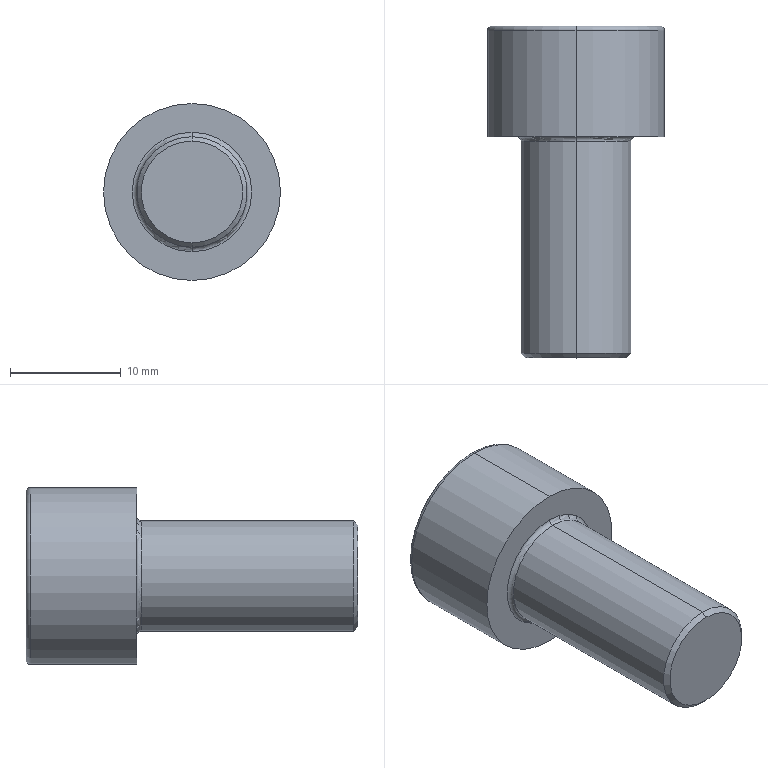Part | STEP file | 1 solid | 20 faces | box 16 x 30 x 16 mm | volume 3301 mm3 | plane 10 | torus 4 | cylinder 4 | cone 2 | commonest cylinder face diameters 10 x2 16 x2
STEP:
#1=CARTESIAN_POINT('',(0.,-20.,-4.6));
#2=VERTEX_POINT('',#1);
#3=CARTESIAN_POINT('',(0.,-20.,4.6));
#4=VERTEX_POINT('',#3);
#5=CARTESIAN_POINT('',(0.,-20.,0.));
#6=DIRECTION('',(0.,-1.,0.));
#7=DIRECTION('',(0.,0.,-1.));
#8=AXIS2_PLACEMENT_3D('',#5,#6,#7);
#9=CIRCLE('',#8,4.6);
#10=EDGE_CURVE('',#2,#4,#9,.T.);
#11=ORIENTED_EDGE('',*,*,#10,.F.);
#12=CARTESIAN_POINT('',(0.,-19.6,-5.));
#13=VERTEX_POINT('',#12);
#14=CARTESIAN_POINT('',(0.,-20.,-4.6));
#15=DIRECTION('',(0.,0.7071,-0.7071));
#16=VECTOR('',#15,1000.);
#17=LINE('',#14,#16);
#18=EDGE_CURVE('',#2,#13,#17,.T.);
#19=ORIENTED_EDGE('',*,*,#18,.T.);
#20=CARTESIAN_POINT('',(0.,-19.6,5.));
#21=VERTEX_POINT('',#20);
#22=CARTESIAN_POINT('',(0.,-19.6,0.));
#23=DIRECTION('',(0.,1.,0.));
#24=DIRECTION('',(0.,0.,-1.));
#25=AXIS2_PLACEMENT_3D('',#22,#23,#24);
#26=CIRCLE('',#25,5.);
#27=EDGE_CURVE('',#21,#13,#26,.T.);
#28=ORIENTED_EDGE('',*,*,#27,.F.);
#29=CARTESIAN_POINT('',(0.,-20.,4.6));
#30=DIRECTION('',(0.,0.7071,0.7071));
#31=VECTOR('',#30,1000.);
#32=LINE('',#29,#31);
#33=EDGE_CURVE('',#4,#21,#32,.T.);
#34=ORIENTED_EDGE('',*,*,#33,.F.);
#35=EDGE_LOOP('',(#11,#19,#28,#34));
#36=FACE_OUTER_BOUND('',#35,.T.);
#37=CARTESIAN_POINT('',(0.,-20.,0.));
#38=DIRECTION('',(0.,1.,0.));
#39=DIRECTION('',(0.,0.,1.));
#40=AXIS2_PLACEMENT_3D('',#37,#38,#39);
#41=CONICAL_SURFACE('',#40,4.6,0.7854);
#42=ADVANCED_FACE('',(#36),#41,.T.);
#43=CARTESIAN_POINT('',(0.,9.6,-8.));
#44=VERTEX_POINT('',#43);
#45=CARTESIAN_POINT('',(0.,9.6,8.));
#46=VERTEX_POINT('',#45);
#47=CARTESIAN_POINT('',(0.,9.6,0.));
#48=DIRECTION('',(0.,-1.,0.));
#49=DIRECTION('',(0.,0.,1.));
#50=AXIS2_PLACEMENT_3D('',#47,#48,#49);
#51=CIRCLE('',#50,8.);
#52=EDGE_CURVE('',#44,#46,#51,.T.);
#53=ORIENTED_EDGE('',*,*,#52,.F.);
#54=CARTESIAN_POINT('',(0.,10.,-7.6));
#55=VERTEX_POINT('',#54);
#56=CARTESIAN_POINT('',(0.,9.6,-7.6));
#57=DIRECTION('',(1.,0.,0.));
#58=DIRECTION('',(0.,0.,-1.));
#59=AXIS2_PLACEMENT_3D('',#56,#57,#58);
#60=CIRCLE('',#59,0.4);
#61=EDGE_CURVE('',#44,#55,#60,.T.);
#62=ORIENTED_EDGE('',*,*,#61,.T.);
#63=CARTESIAN_POINT('',(0.,10.,7.6));
#64=VERTEX_POINT('',#63);
#65=CARTESIAN_POINT('',(0.,10.,0.));
#66=DIRECTION('',(0.,1.,0.));
#67=DIRECTION('',(0.,0.,1.));
#68=AXIS2_PLACEMENT_3D('',#65,#66,#67);
#69=CIRCLE('',#68,7.6);
#70=EDGE_CURVE('',#64,#55,#69,.T.);
#71=ORIENTED_EDGE('',*,*,#70,.F.);
#72=CARTESIAN_POINT('',(0.,9.6,7.6));
#73=DIRECTION('',(-1.,0.,0.));
#74=DIRECTION('',(0.,0.,1.));
#75=AXIS2_PLACEMENT_3D('',#72,#73,#74);
#76=CIRCLE('',#75,0.4);
#77=EDGE_CURVE('',#46,#64,#76,.T.);
#78=ORIENTED_EDGE('',*,*,#77,.F.);
#79=EDGE_LOOP('',(#53,#62,#71,#78));
#80=FACE_OUTER_BOUND('',#79,.T.);
#81=CARTESIAN_POINT('',(0.,9.6,0.));
#82=DIRECTION('',(0.,1.,0.));
#83=DIRECTION('',(0.,0.,1.));
#84=AXIS2_PLACEMENT_3D('',#81,#82,#83);
#85=TOROIDAL_SURFACE('',#84,7.6,0.4);
#86=ADVANCED_FACE('',(#80),#85,.T.);
#87=CARTESIAN_POINT('',(0.,-0.4,5.));
#88=VERTEX_POINT('',#87);
#89=CARTESIAN_POINT('',(0.,-0.4,-5.));
#90=VERTEX_POINT('',#89);
#91=CARTESIAN_POINT('',(0.,-0.4,0.));
#92=DIRECTION('',(0.,-1.,0.));
#93=DIRECTION('',(0.,0.,-1.));
#94=AXIS2_PLACEMENT_3D('',#91,#92,#93);
#95=CIRCLE('',#94,5.);
#96=EDGE_CURVE('',#88,#90,#95,.T.);
#97=ORIENTED_EDGE('',*,*,#96,.F.);
#98=CARTESIAN_POINT('',(0.,0.,5.4));
#99=VERTEX_POINT('',#98);
#100=CARTESIAN_POINT('',(0.,-0.4,5.4));
#101=DIRECTION('',(1.,0.,0.));
#102=DIRECTION('',(0.,0.,-1.));
#103=AXIS2_PLACEMENT_3D('',#100,#101,#102);
#104=CIRCLE('',#103,0.4);
#105=EDGE_CURVE('',#88,#99,#104,.T.);
#106=ORIENTED_EDGE('',*,*,#105,.T.);
#107=CARTESIAN_POINT('',(0.,0.,-5.4));
#108=VERTEX_POINT('',#107);
#109=CARTESIAN_POINT('',(0.,0.,0.));
#110=DIRECTION('',(0.,1.,0.));
#111=DIRECTION('',(0.,0.,-1.));
#112=AXIS2_PLACEMENT_3D('',#109,#110,#111);
#113=CIRCLE('',#112,5.4);
#114=EDGE_CURVE('',#108,#99,#113,.T.);
#115=ORIENTED_EDGE('',*,*,#114,.F.);
#116=CARTESIAN_POINT('',(0.,-0.4,-5.4));
#117=DIRECTION('',(-1.,0.,0.));
#118=DIRECTION('',(0.,0.,1.));
#119=AXIS2_PLACEMENT_3D('',#116,#117,#118);
#120=CIRCLE('',#119,0.4);
#121=EDGE_CURVE('',#90,#108,#120,.T.);
#122=ORIENTED_EDGE('',*,*,#121,.F.);
#123=EDGE_LOOP('',(#97,#106,#115,#122));
#124=FACE_OUTER_BOUND('',#123,.T.);
#125=CARTESIAN_POINT('',(0.,-0.4,0.));
#126=DIRECTION('',(0.,-1.,0.));
#127=DIRECTION('',(0.,0.,-1.));
#128=AXIS2_PLACEMENT_3D('',#125,#126,#127);
#129=TOROIDAL_SURFACE('',#128,5.4,0.4);
#130=ADVANCED_FACE('',(#124),#129,.F.);
#131=CARTESIAN_POINT('',(0.,-0.4,0.));
#132=DIRECTION('',(0.,-1.,0.));
#133=DIRECTION('',(0.,0.,-1.));
#134=AXIS2_PLACEMENT_3D('',#131,#132,#133);
#135=CIRCLE('',#134,5.);
#136=EDGE_CURVE('',#90,#88,#135,.T.);
#137=ORIENTED_EDGE('',*,*,#136,.T.);
#138=CARTESIAN_POINT('',(0.,0.,5.));
#139=DIRECTION('',(0.,-1.,0.));
#140=VECTOR('',#139,1000.);
#141=LINE('',#138,#140);
#142=EDGE_CURVE('',#88,#21,#141,.T.);
#143=ORIENTED_EDGE('',*,*,#142,.T.);
#144=ORIENTED_EDGE('',*,*,#27,.T.);
#145=CARTESIAN_POINT('',(0.,0.,-5.));
#146=DIRECTION('',(0.,-1.,0.));
#147=VECTOR('',#146,1000.);
#148=LINE('',#145,#147);
#149=EDGE_CURVE('',#90,#13,#148,.T.);
#150=ORIENTED_EDGE('',*,*,#149,.F.);
#151=EDGE_LOOP('',(#137,#143,#144,#150));
#152=FACE_OUTER_BOUND('',#151,.T.);
#153=CARTESIAN_POINT('',(0.,0.,0.));
#154=DIRECTION('',(0.,-1.,0.));
#155=DIRECTION('',(0.,0.,-1.));
#156=AXIS2_PLACEMENT_3D('',#153,#154,#155);
#157=CYLINDRICAL_SURFACE('',#156,5.);
#158=ADVANCED_FACE('',(#152),#157,.T.);
#159=ORIENTED_EDGE('',*,*,#52,.T.);
#160=CARTESIAN_POINT('',(0.,0.,8.));
#161=VERTEX_POINT('',#160);
#162=CARTESIAN_POINT('',(0.,0.,8.));
#163=DIRECTION('',(0.,-1.,0.));
#164=VECTOR('',#163,1000.);
#165=LINE('',#162,#164);
#166=EDGE_CURVE('',#46,#161,#165,.T.);
#167=ORIENTED_EDGE('',*,*,#166,.T.);
#168=CARTESIAN_POINT('',(0.,0.,-8.));
#169=VERTEX_POINT('',#168);
#170=CARTESIAN_POINT('',(0.,0.,0.));
#171=DIRECTION('',(0.,-1.,0.));
#172=DIRECTION('',(0.,0.,-1.));
#173=AXIS2_PLACEMENT_3D('',#170,#171,#172);
#174=CIRCLE('',#173,8.);
#175=EDGE_CURVE('',#169,#161,#174,.T.);
#176=ORIENTED_EDGE('',*,*,#175,.F.);
#177=CARTESIAN_POINT('',(0.,0.,-8.));
#178=DIRECTION('',(0.,-1.,0.));
#179=VECTOR('',#178,1000.);
#180=LINE('',#177,#179);
#181=EDGE_CURVE('',#44,#169,#180,.T.);
#182=ORIENTED_EDGE('',*,*,#181,.F.);
#183=EDGE_LOOP('',(#159,#167,#176,#182));
#184=FACE_OUTER_BOUND('',#183,.T.);
#185=CARTESIAN_POINT('',(0.,0.,0.));
#186=DIRECTION('',(0.,-1.,0.));
#187=DIRECTION('',(0.,0.,-1.));
#188=AXIS2_PLACEMENT_3D('',#185,#186,#187);
#189=CYLINDRICAL_SURFACE('',#188,8.);
#190=ADVANCED_FACE('',(#184),#189,.T.);
#191=ORIENTED_EDGE('',*,*,#70,.T.);
#192=CARTESIAN_POINT('',(0.,10.,0.));
#193=DIRECTION('',(0.,1.,0.));
#194=DIRECTION('',(0.,0.,1.));
#195=AXIS2_PLACEMENT_3D('',#192,#193,#194);
#196=CIRCLE('',#195,7.6);
#197=EDGE_CURVE('',#55,#64,#196,.T.);
#198=ORIENTED_EDGE('',*,*,#197,.T.);
#199=EDGE_LOOP('',(#191,#198));
#200=FACE_OUTER_BOUND('',#199,.T.);
#201=CARTESIAN_POINT('',(0.,10.,-4.619));
#202=VERTEX_POINT('',#201);
#203=CARTESIAN_POINT('',(-4.,10.,-2.309));
#204=VERTEX_POINT('',#203);
#205=CARTESIAN_POINT('',(0.,10.,-4.619));
#206=DIRECTION('',(-0.866,0.,0.5));
#207=VECTOR('',#206,1000.);
#208=LINE('',#205,#207);
#209=EDGE_CURVE('',#202,#204,#208,.T.);
#210=ORIENTED_EDGE('',*,*,#209,.F.);
#211=CARTESIAN_POINT('',(4.,10.,-2.309));
#212=VERTEX_POINT('',#211);
#213=CARTESIAN_POINT('',(4.,10.,-2.309));
#214=DIRECTION('',(-0.866,0.,-0.5));
#215=VECTOR('',#214,1000.);
#216=LINE('',#213,#215);
#217=EDGE_CURVE('',#212,#202,#216,.T.);
#218=ORIENTED_EDGE('',*,*,#217,.F.);
#219=CARTESIAN_POINT('',(4.,10.,2.309));
#220=VERTEX_POINT('',#219);
#221=CARTESIAN_POINT('',(4.,10.,2.309));
#222=DIRECTION('',(0.,0.,-1.));
#223=VECTOR('',#222,1000.);
#224=LINE('',#221,#223);
#225=EDGE_CURVE('',#220,#212,#224,.T.);
#226=ORIENTED_EDGE('',*,*,#225,.F.);
#227=CARTESIAN_POINT('',(0.,10.,4.619));
#228=VERTEX_POINT('',#227);
#229=CARTESIAN_POINT('',(0.,10.,4.619));
#230=DIRECTION('',(0.866,0.,-0.5));
#231=VECTOR('',#230,1000.);
#232=LINE('',#229,#231);
#233=EDGE_CURVE('',#228,#220,#232,.T.);
#234=ORIENTED_EDGE('',*,*,#233,.F.);
#235=CARTESIAN_POINT('',(-4.,10.,2.309));
#236=VERTEX_POINT('',#235);
#237=CARTESIAN_POINT('',(-4.,10.,2.309));
#238=DIRECTION('',(0.866,0.,0.5));
#239=VECTOR('',#238,1000.);
#240=LINE('',#237,#239);
#241=EDGE_CURVE('',#236,#228,#240,.T.);
#242=ORIENTED_EDGE('',*,*,#241,.F.);
#243=CARTESIAN_POINT('',(-4.,10.,-2.309));
#244=DIRECTION('',(0.,0.,1.));
#245=VECTOR('',#244,1000.);
#246=LINE('',#243,#245);
#247=EDGE_CURVE('',#204,#236,#246,.T.);
#248=ORIENTED_EDGE('',*,*,#247,.F.);
#249=EDGE_LOOP('',(#210,#218,#226,#234,#242,#248));
#250=FACE_BOUND('',#249,.T.);
#251=CARTESIAN_POINT('',(0.,10.,0.));
#252=DIRECTION('',(0.,1.,0.));
#253=DIRECTION('',(0.,0.,1.));
#254=AXIS2_PLACEMENT_3D('',#251,#252,#253);
#255=PLANE('',#254);
#256=ADVANCED_FACE('',(#200,#250),#255,.T.);
#257=ORIENTED_EDGE('',*,*,#166,.F.);
#258=CARTESIAN_POINT('',(0.,9.6,0.));
#259=DIRECTION('',(0.,-1.,0.));
#260=DIRECTION('',(0.,0.,1.));
#261=AXIS2_PLACEMENT_3D('',#258,#259,#260);
#262=CIRCLE('',#261,8.);
#263=EDGE_CURVE('',#46,#44,#262,.T.);
#264=ORIENTED_EDGE('',*,*,#263,.T.);
#265=ORIENTED_EDGE('',*,*,#181,.T.);
#266=CARTESIAN_POINT('',(0.,0.,0.));
#267=DIRECTION('',(0.,-1.,0.));
#268=DIRECTION('',(0.,0.,-1.));
#269=AXIS2_PLACEMENT_3D('',#266,#267,#268);
#270=CIRCLE('',#269,8.);
#271=EDGE_CURVE('',#161,#169,#270,.T.);
#272=ORIENTED_EDGE('',*,*,#271,.F.);
#273=EDGE_LOOP('',(#257,#264,#265,#272));
#274=FACE_OUTER_BOUND('',#273,.T.);
#275=CARTESIAN_POINT('',(0.,0.,0.));
#276=DIRECTION('',(0.,-1.,0.));
#277=DIRECTION('',(0.,0.,-1.));
#278=AXIS2_PLACEMENT_3D('',#275,#276,#277);
#279=CYLINDRICAL_SURFACE('',#278,8.);
#280=ADVANCED_FACE('',(#274),#279,.T.);
#281=ORIENTED_EDGE('',*,*,#114,.T.);
#282=CARTESIAN_POINT('',(0.,0.,0.));
#283=DIRECTION('',(0.,1.,0.));
#284=DIRECTION('',(0.,0.,-1.));
#285=AXIS2_PLACEMENT_3D('',#282,#283,#284);
#286=CIRCLE('',#285,5.4);
#287=EDGE_CURVE('',#99,#108,#286,.T.);
#288=ORIENTED_EDGE('',*,*,#287,.T.);
#289=EDGE_LOOP('',(#281,#288));
#290=FACE_BOUND('',#289,.T.);
#291=ORIENTED_EDGE('',*,*,#175,.T.);
#292=ORIENTED_EDGE('',*,*,#271,.T.);
#293=EDGE_LOOP('',(#291,#292));
#294=FACE_OUTER_BOUND('',#293,.T.);
#295=CARTESIAN_POINT('',(8.,0.,0.));
#296=DIRECTION('',(0.,-1.,0.));
#297=DIRECTION('',(0.,0.,-1.));
#298=AXIS2_PLACEMENT_3D('',#295,#296,#297);
#299=PLANE('',#298);
#300=ADVANCED_FACE('',(#290,#294),#299,.T.);
#301=ORIENTED_EDGE('',*,*,#142,.F.);
#302=ORIENTED_EDGE('',*,*,#96,.T.);
#303=ORIENTED_EDGE('',*,*,#149,.T.);
#304=CARTESIAN_POINT('',(0.,-19.6,0.));
#305=DIRECTION('',(0.,1.,0.));
#306=DIRECTION('',(0.,0.,-1.));
#307=AXIS2_PLACEMENT_3D('',#304,#305,#306);
#308=CIRCLE('',#307,5.);
#309=EDGE_CURVE('',#13,#21,#308,.T.);
#310=ORIENTED_EDGE('',*,*,#309,.T.);
#311=EDGE_LOOP('',(#301,#302,#303,#310));
#312=FACE_OUTER_BOUND('',#311,.T.);
#313=CARTESIAN_POINT('',(0.,0.,0.));
#314=DIRECTION('',(0.,-1.,0.));
#315=DIRECTION('',(0.,0.,-1.));
#316=AXIS2_PLACEMENT_3D('',#313,#314,#315);
#317=CYLINDRICAL_SURFACE('',#316,5.);
#318=ADVANCED_FACE('',(#312),#317,.T.);
#319=CARTESIAN_POINT('',(0.,-20.,0.));
#320=DIRECTION('',(0.,-1.,0.));
#321=DIRECTION('',(0.,0.,-1.));
#322=AXIS2_PLACEMENT_3D('',#319,#320,#321);
#323=CIRCLE('',#322,4.6);
#324=EDGE_CURVE('',#4,#2,#323,.T.);
#325=ORIENTED_EDGE('',*,*,#324,.T.);
#326=ORIENTED_EDGE('',*,*,#10,.T.);
#327=EDGE_LOOP('',(#325,#326));
#328=FACE_OUTER_BOUND('',#327,.T.);
#329=CARTESIAN_POINT('',(5.,-20.,0.));
#330=DIRECTION('',(0.,-1.,0.));
#331=DIRECTION('',(0.,0.,-1.));
#332=AXIS2_PLACEMENT_3D('',#329,#330,#331);
#333=PLANE('',#332);
#334=ADVANCED_FACE('',(#328),#333,.T.);
#335=ORIENTED_EDGE('',*,*,#209,.T.);
#336=CARTESIAN_POINT('',(-4.,5.,-2.309));
#337=VERTEX_POINT('',#336);
#338=CARTESIAN_POINT('',(-4.,5.,-2.309));
#339=DIRECTION('',(0.,1.,0.));
#340=VECTOR('',#339,1000.);
#341=LINE('',#338,#340);
#342=EDGE_CURVE('',#337,#204,#341,.T.);
#343=ORIENTED_EDGE('',*,*,#342,.F.);
#344=CARTESIAN_POINT('',(0.,5.,-4.619));
#345=VERTEX_POINT('',#344);
#346=CARTESIAN_POINT('',(0.,5.,-4.619));
#347=DIRECTION('',(-0.866,0.,0.5));
#348=VECTOR('',#347,1000.);
#349=LINE('',#346,#348);
#350=EDGE_CURVE('',#345,#337,#349,.T.);
#351=ORIENTED_EDGE('',*,*,#350,.F.);
#352=CARTESIAN_POINT('',(0.,5.,-4.619));
#353=DIRECTION('',(0.,1.,0.));
#354=VECTOR('',#353,1000.);
#355=LINE('',#352,#354);
#356=EDGE_CURVE('',#345,#202,#355,.T.);
#357=ORIENTED_EDGE('',*,*,#356,.T.);
#358=EDGE_LOOP('',(#335,#343,#351,#357));
#359=FACE_OUTER_BOUND('',#358,.T.);
#360=CARTESIAN_POINT('',(0.,5.,-4.619));
#361=DIRECTION('',(-0.5,0.,-0.866));
#362=DIRECTION('',(-0.866,0.,0.5));
#363=AXIS2_PLACEMENT_3D('',#360,#361,#362);
#364=PLANE('',#363);
#365=ADVANCED_FACE('',(#359),#364,.F.);
#366=ORIENTED_EDGE('',*,*,#217,.T.);
#367=ORIENTED_EDGE('',*,*,#356,.F.);
#368=CARTESIAN_POINT('',(4.,5.,-2.309));
#369=VERTEX_POINT('',#368);
#370=CARTESIAN_POINT('',(4.,5.,-2.309));
#371=DIRECTION('',(-0.866,0.,-0.5));
#372=VECTOR('',#371,1000.);
#373=LINE('',#370,#372);
#374=EDGE_CURVE('',#369,#345,#373,.T.);
#375=ORIENTED_EDGE('',*,*,#374,.F.);
#376=CARTESIAN_POINT('',(4.,5.,-2.309));
#377=DIRECTION('',(0.,1.,0.));
#378=VECTOR('',#377,1000.);
#379=LINE('',#376,#378);
#380=EDGE_CURVE('',#369,#212,#379,.T.);
#381=ORIENTED_EDGE('',*,*,#380,.T.);
#382=EDGE_LOOP('',(#366,#367,#375,#381));
#383=FACE_OUTER_BOUND('',#382,.T.);
#384=CARTESIAN_POINT('',(4.,5.,-2.309));
#385=DIRECTION('',(0.5,0.,-0.866));
#386=DIRECTION('',(-0.866,0.,-0.5));
#387=AXIS2_PLACEMENT_3D('',#384,#385,#386);
#388=PLANE('',#387);
#389=ADVANCED_FACE('',(#383),#388,.F.);
#390=ORIENTED_EDGE('',*,*,#225,.T.);
#391=ORIENTED_EDGE('',*,*,#380,.F.);
#392=CARTESIAN_POINT('',(4.,5.,2.309));
#393=VERTEX_POINT('',#392);
#394=CARTESIAN_POINT('',(4.,5.,2.309));
#395=DIRECTION('',(0.,0.,-1.));
#396=VECTOR('',#395,1000.);
#397=LINE('',#394,#396);
#398=EDGE_CURVE('',#393,#369,#397,.T.);
#399=ORIENTED_EDGE('',*,*,#398,.F.);
#400=CARTESIAN_POINT('',(4.,5.,2.309));
#401=DIRECTION('',(0.,1.,0.));
#402=VECTOR('',#401,1000.);
#403=LINE('',#400,#402);
#404=EDGE_CURVE('',#393,#220,#403,.T.);
#405=ORIENTED_EDGE('',*,*,#404,.T.);
#406=EDGE_LOOP('',(#390,#391,#399,#405));
#407=FACE_OUTER_BOUND('',#406,.T.);
#408=CARTESIAN_POINT('',(4.,5.,2.309));
#409=DIRECTION('',(1.,0.,0.));
#410=DIRECTION('',(0.,0.,-1.));
#411=AXIS2_PLACEMENT_3D('',#408,#409,#410);
#412=PLANE('',#411);
#413=ADVANCED_FACE('',(#407),#412,.F.);
#414=ORIENTED_EDGE('',*,*,#233,.T.);
#415=ORIENTED_EDGE('',*,*,#404,.F.);
#416=CARTESIAN_POINT('',(0.,5.,4.619));
#417=VERTEX_POINT('',#416);
#418=CARTESIAN_POINT('',(0.,5.,4.619));
#419=DIRECTION('',(0.866,0.,-0.5));
#420=VECTOR('',#419,1000.);
#421=LINE('',#418,#420);
#422=EDGE_CURVE('',#417,#393,#421,.T.);
#423=ORIENTED_EDGE('',*,*,#422,.F.);
#424=CARTESIAN_POINT('',(0.,5.,4.619));
#425=DIRECTION('',(0.,1.,0.));
#426=VECTOR('',#425,1000.);
#427=LINE('',#424,#426);
#428=EDGE_CURVE('',#417,#228,#427,.T.);
#429=ORIENTED_EDGE('',*,*,#428,.T.);
#430=EDGE_LOOP('',(#414,#415,#423,#429));
#431=FACE_OUTER_BOUND('',#430,.T.);
#432=CARTESIAN_POINT('',(0.,5.,4.619));
#433=DIRECTION('',(0.5,0.,0.866));
#434=DIRECTION('',(0.866,0.,-0.5));
#435=AXIS2_PLACEMENT_3D('',#432,#433,#434);
#436=PLANE('',#435);
#437=ADVANCED_FACE('',(#431),#436,.F.);
#438=ORIENTED_EDGE('',*,*,#241,.T.);
#439=ORIENTED_EDGE('',*,*,#428,.F.);
#440=CARTESIAN_POINT('',(-4.,5.,2.309));
#441=VERTEX_POINT('',#440);
#442=CARTESIAN_POINT('',(-4.,5.,2.309));
#443=DIRECTION('',(0.866,0.,0.5));
#444=VECTOR('',#443,1000.);
#445=LINE('',#442,#444);
#446=EDGE_CURVE('',#441,#417,#445,.T.);
#447=ORIENTED_EDGE('',*,*,#446,.F.);
#448=CARTESIAN_POINT('',(-4.,5.,2.309));
#449=DIRECTION('',(0.,1.,0.));
#450=VECTOR('',#449,1000.);
#451=LINE('',#448,#450);
#452=EDGE_CURVE('',#441,#236,#451,.T.);
#453=ORIENTED_EDGE('',*,*,#452,.T.);
#454=EDGE_LOOP('',(#438,#439,#447,#453));
#455=FACE_OUTER_BOUND('',#454,.T.);
#456=CARTESIAN_POINT('',(-4.,5.,2.309));
#457=DIRECTION('',(-0.5,0.,0.866));
#458=DIRECTION('',(0.866,0.,0.5));
#459=AXIS2_PLACEMENT_3D('',#456,#457,#458);
#460=PLANE('',#459);
#461=ADVANCED_FACE('',(#455),#460,.F.);
#462=ORIENTED_EDGE('',*,*,#247,.T.);
#463=ORIENTED_EDGE('',*,*,#452,.F.);
#464=CARTESIAN_POINT('',(-4.,5.,-2.309));
#465=DIRECTION('',(0.,0.,1.));
#466=VECTOR('',#465,1000.);
#467=LINE('',#464,#466);
#468=EDGE_CURVE('',#337,#441,#467,.T.);
#469=ORIENTED_EDGE('',*,*,#468,.F.);
#470=ORIENTED_EDGE('',*,*,#342,.T.);
#471=EDGE_LOOP('',(#462,#463,#469,#470));
#472=FACE_OUTER_BOUND('',#471,.T.);
#473=CARTESIAN_POINT('',(-4.,5.,-2.309));
#474=DIRECTION('',(-1.,0.,0.));
#475=DIRECTION('',(0.,0.,1.));
#476=AXIS2_PLACEMENT_3D('',#473,#474,#475);
#477=PLANE('',#476);
#478=ADVANCED_FACE('',(#472),#477,.F.);
#479=ORIENTED_EDGE('',*,*,#350,.T.);
#480=ORIENTED_EDGE('',*,*,#468,.T.);
#481=ORIENTED_EDGE('',*,*,#446,.T.);
#482=ORIENTED_EDGE('',*,*,#422,.T.);
#483=ORIENTED_EDGE('',*,*,#398,.T.);
#484=ORIENTED_EDGE('',*,*,#374,.T.);
#485=EDGE_LOOP('',(#479,#480,#481,#482,#483,#484));
#486=FACE_OUTER_BOUND('',#485,.T.);
#487=CARTESIAN_POINT('',(0.,5.,0.));
#488=DIRECTION('',(0.,1.,0.));
#489=DIRECTION('',(0.,0.,1.));
#490=AXIS2_PLACEMENT_3D('',#487,#488,#489);
#491=PLANE('',#490);
#492=ADVANCED_FACE('',(#486),#491,.T.);
#493=ORIENTED_EDGE('',*,*,#105,.F.);
#494=ORIENTED_EDGE('',*,*,#136,.F.);
#495=ORIENTED_EDGE('',*,*,#121,.T.);
#496=ORIENTED_EDGE('',*,*,#287,.F.);
#497=EDGE_LOOP('',(#493,#494,#495,#496));
#498=FACE_OUTER_BOUND('',#497,.T.);
#499=CARTESIAN_POINT('',(0.,-0.4,0.));
#500=DIRECTION('',(0.,-1.,0.));
#501=DIRECTION('',(0.,0.,-1.));
#502=AXIS2_PLACEMENT_3D('',#499,#500,#501);
#503=TOROIDAL_SURFACE('',#502,5.4,0.4);
#504=ADVANCED_FACE('',(#498),#503,.F.);
#505=ORIENTED_EDGE('',*,*,#61,.F.);
#506=ORIENTED_EDGE('',*,*,#263,.F.);
#507=ORIENTED_EDGE('',*,*,#77,.T.);
#508=ORIENTED_EDGE('',*,*,#197,.F.);
#509=EDGE_LOOP('',(#505,#506,#507,#508));
#510=FACE_OUTER_BOUND('',#509,.T.);
#511=CARTESIAN_POINT('',(0.,9.6,0.));
#512=DIRECTION('',(0.,1.,0.));
#513=DIRECTION('',(0.,0.,1.));
#514=AXIS2_PLACEMENT_3D('',#511,#512,#513);
#515=TOROIDAL_SURFACE('',#514,7.6,0.4);
#516=ADVANCED_FACE('',(#510),#515,.T.);
#517=ORIENTED_EDGE('',*,*,#18,.F.);
#518=ORIENTED_EDGE('',*,*,#324,.F.);
#519=ORIENTED_EDGE('',*,*,#33,.T.);
#520=ORIENTED_EDGE('',*,*,#309,.F.);
#521=EDGE_LOOP('',(#517,#518,#519,#520));
#522=FACE_OUTER_BOUND('',#521,.T.);
#523=CARTESIAN_POINT('',(0.,-20.,0.));
#524=DIRECTION('',(0.,1.,0.));
#525=DIRECTION('',(0.,0.,1.));
#526=AXIS2_PLACEMENT_3D('',#523,#524,#525);
#527=CONICAL_SURFACE('',#526,4.6,0.7854);
#528=ADVANCED_FACE('',(#522),#527,.T.);
#529=CLOSED_SHELL('',(#42,#86,#130,#158,#190,#256,#280,#300,#318,#334,#365,#389,#413,#437,#461,#478,#492,#504,#516,#528));
#530=MANIFOLD_SOLID_BREP('',#529);
#531=CARTESIAN_POINT('',(0.,0.,0.));
#532=DIRECTION('',(0.,0.,1.));
#533=DIRECTION('',(1.,0.,0.));
#534=AXIS2_PLACEMENT_3D('',#531,#532,#533);
#535=(LENGTH_UNIT()NAMED_UNIT(*)SI_UNIT(.MILLI.,.METRE.));
#536=UNCERTAINTY_MEASURE_WITH_UNIT(LENGTH_MEASURE(0.00001),#535,'','');
#537=(NAMED_UNIT(*)PLANE_ANGLE_UNIT()SI_UNIT($,.RADIAN.));
#538=(NAMED_UNIT(*)SI_UNIT($,.STERADIAN.)SOLID_ANGLE_UNIT());
#539=(GEOMETRIC_REPRESENTATION_CONTEXT(3)GLOBAL_UNCERTAINTY_ASSIGNED_CONTEXT((#536))GLOBAL_UNIT_ASSIGNED_CONTEXT((#535,#537,#538))REPRESENTATION_CONTEXT('',''));
#540=ADVANCED_BREP_SHAPE_REPRESENTATION('',(#530,#534),#539);